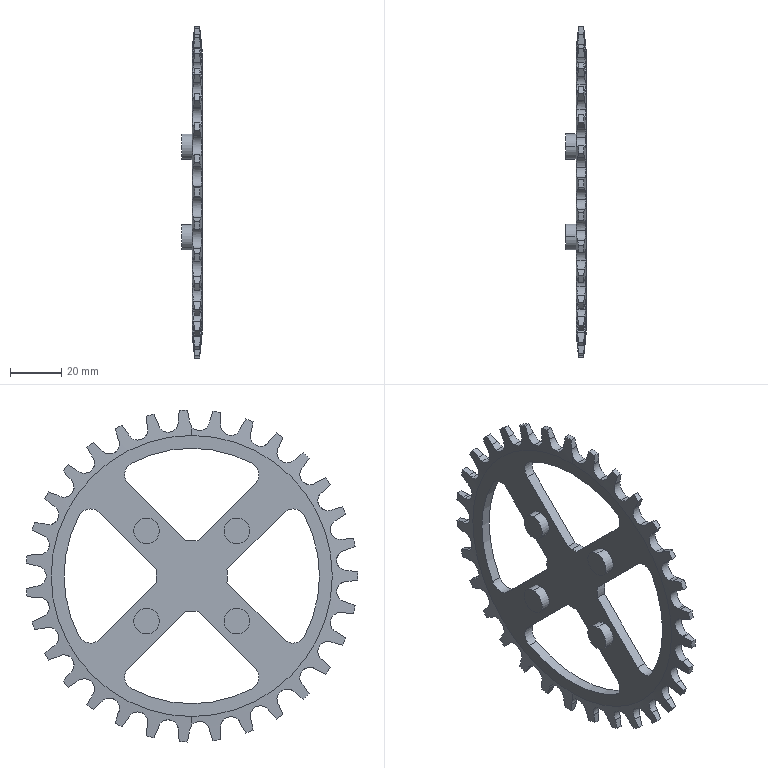Part | STEP file | Front gears middle | 1 solid | 185 faces | box 8 x 129.807 x 129.955 mm | volume 26124 mm3 | cylinder 105 | plane 76 | cone 4 | commonest cylinder face diameters 8 x46 130 x31 10 x18 28 x5 100 x5